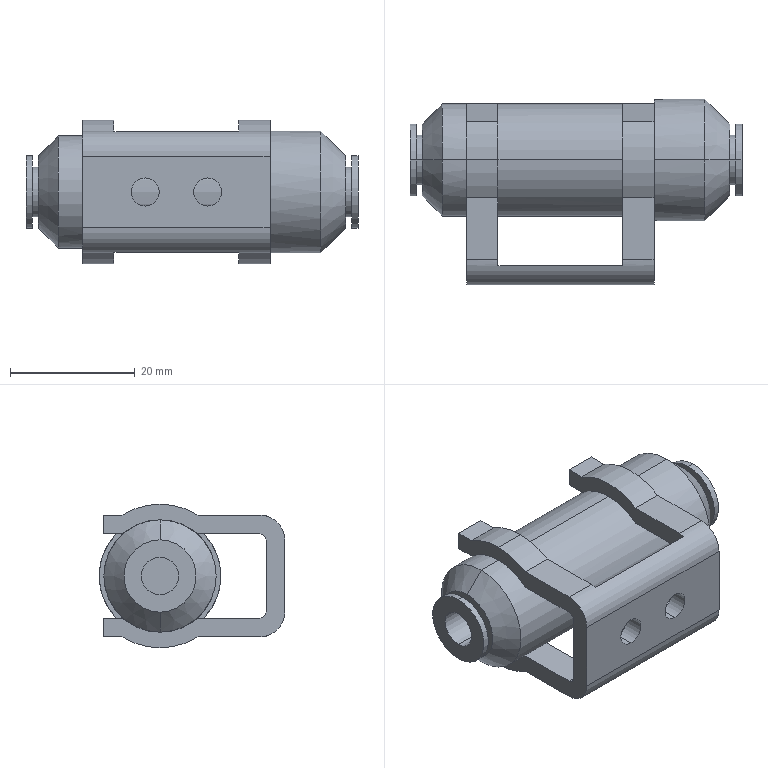Part | SolidWorks | features ICE 8, Revolution 1 | 1 solid | 74 faces | box 53.2 x 29.75 x 23 mm | volume 14418 mm3 | plane 38 | cylinder 32 | cone 4 | commonest cylinder face diameters 8 x6 23 x6 2 x4 4.5 x4 6 x4 11.6 x4